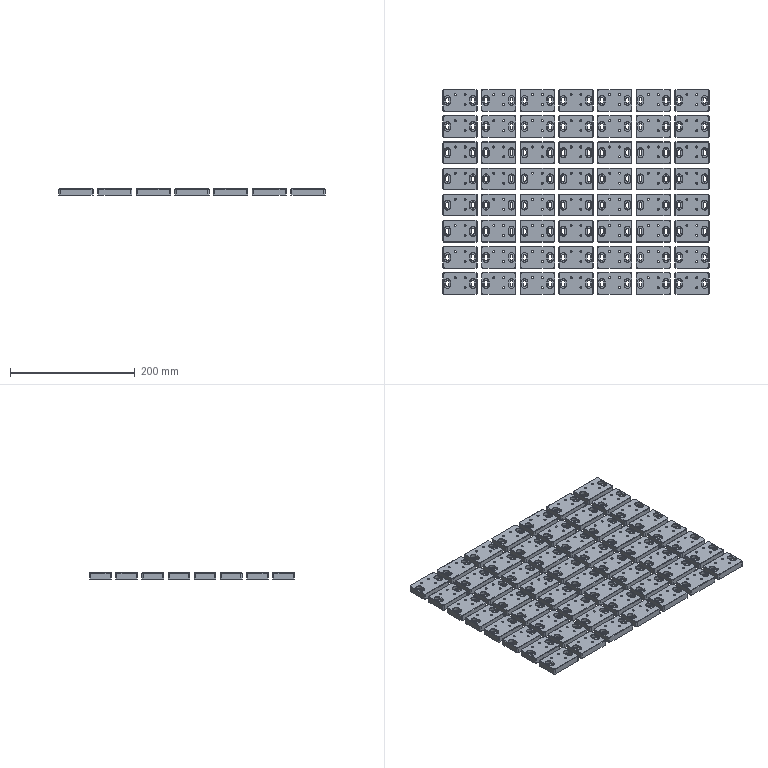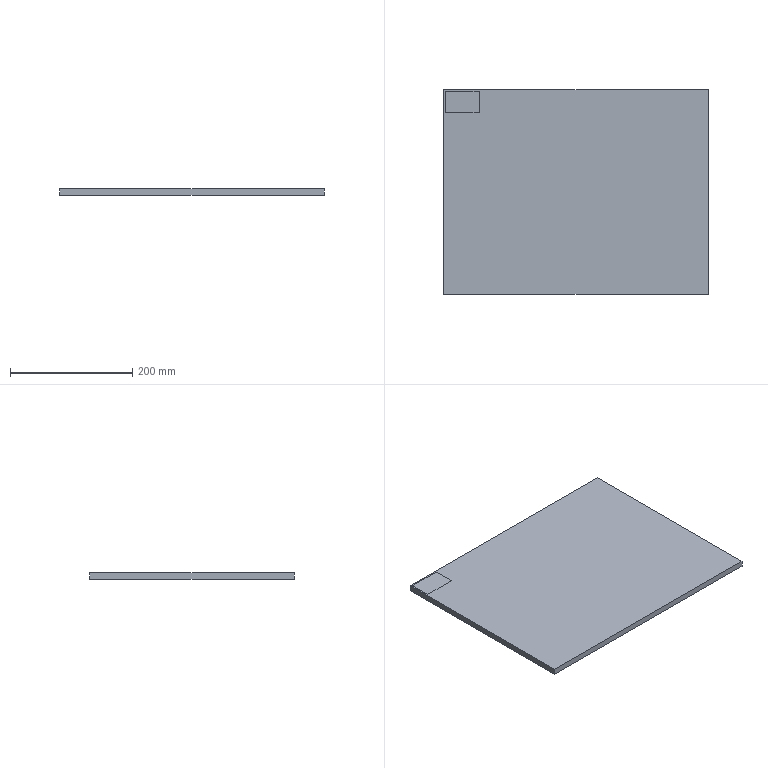CAM job | NX | 3-axis milling, drilling | part box 427 x 329 x 10 mm | stock box 433 x 335 x 10 mm
Tools:
number,name,description,diameter,corner_radius,flute_length,length,flutes
4,D4,Milling Tool-5 Parameters,4.0,0.0,50.0,75.0,2
6,D6,Milling Tool-5 Parameters,6.0,0.0,50.0,75.0,2
2,D4A45,Milling Tool-5 Parameters,4.0,0.0,2.0,2.0,2
13,3.3ZT,Drilling Tool,3.1,0.0,35.0,50.0,2
Operations:
program,operation,operation_type,tool,method,geometry_group,spindle_rpm,surface_speed,feed_per_tooth,feed_cut,feed_plunge,cut_length_mm,path_length_mm,cut_time_min,machine_time_min
1吸,ZLEVEL_PROFILE_COPY_COPY_1_COPY_COPY_COPY,ZLevelMilling,D4,METHOD,A,9500.0,179.0,0.0737,1400.0,1000.0,28898.541,40612.026,21.739,22.91
1吸,ZLEVEL_PROFILE_COPY_COPY_1_COPY,ZLevelMilling,D6,METHOD,A,9500.0,179.0,0.1158,2200.0,1000.0,223337.684,235016.865,102.676,103.844
1吸,ZLEVEL_PROFILE_1_COPY_1_COPY_COPY,ZLevelMilling,D4A45,METHOD,A,9500.0,179.0,0.0526,1000.0,100.0,14371.392,51798.539,14.371,18.114
1吸,ZLEVEL_PROFILE_COPY_COPY_COPY_COPY_COPY,ZLevelMilling,D6,MILL_FINISH,A,9500.0,119.0,0.0632,1200.0,1000.0,11180.083,28786.383,9.336,11.097
2,DRILLING_COPY,Operation,D4A45,METHOD,B,5000.0,62.0,0.025,250.0,0.0,12.0,122.361,0.048,0.059
2,DRILLING_COPY_COPY_COPY_COPY_COPY_COPY_1,Operation,3.3ZT,METHOD,B,1910.0,21.0,0.0471,180.0,0.0,46.294,190.949,0.2572,0.2717
2,ZLEVEL_PROFILE_COPY_COPY_1_COPY_COPY,ZLevelMilling,D6,METHOD,B,9500.0,179.0,0.1158,2200.0,1000.0,537.637,703.182,0.2861,0.3026
2,ZLEVEL_PROFILE_COPY_COPY_COPY_COPY_COPY_COPY,ZLevelMilling,D6,MILL_FINISH,B,9500.0,119.0,0.0632,1200.0,1000.0,52.797,230.924,0.0448,0.0626
2,ZLEVEL_PROFILE_1_COPY_1_COPY_COPY_COPY,ZLevelMilling,D4A45,METHOD,B,9500.0,179.0,0.0526,1000.0,100.0,291.441,768.561,0.2914,0.3392